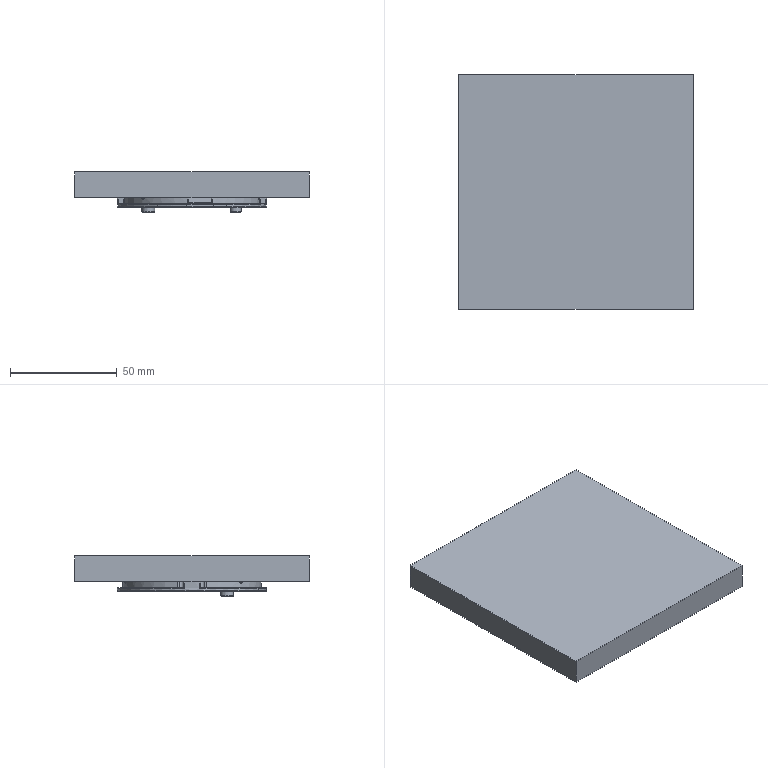NC program | NX | posted with a generic post | part box 110 x 110 x 18.8 mm
Lines 1 to 1769 of 9447:
N10 G17 G21 G94 G90
(FLOOR_WALL , TOOL : D63)
N12 T03 M6
N14 G54
N16 G17 G0 G90 X-77.5 Y42.997 S6500 M3
N18 G43 Z30. H3
N20 Z3.
N22 G94 G1 Z0. F1250.
N24 X-74.5
N26 X74.5
N28 Y12.599
N30 X-74.5
N32 Y-17.8
N34 X74.5
N36 X77.5
N38 Z3.
N40 G0 Z30.
N42 M5
(CAVITY_MILL , TOOL : D10)
N44 T04 M6
N46 G54
N48 G17 G0 G90 X-49.996 Y-4.33 S9500 M3
N50 G43 Z30. H4
N52 Z0.52
N54 G94 G1 Z-0.98 F1000.
N56 X-43.996 Y-0.866
N58 G3 X-43.496 Y0. R1.
N60 G1 Y43.007 F3000.
N62 G2 X-43.007 Y43.496 R0.489
N64 G1 X43.007
N66 G2 X43.496 Y43.007 R0.489
N68 G1 Y-43.007
N70 G2 X43.007 Y-43.496 R0.489
N72 G1 X-43.007
N74 G2 X-43.496 Y-43.007 R0.489
N76 G1 Y0.
N78 X-37.496
N80 Y37.496
N82 X37.496
N84 Y-37.496
N86 X-37.496
N88 Y0.
N90 X-31.496
N92 Y31.496
N94 X31.496
N96 Y-31.496
N98 X-31.496
N100 Y0.
N102 X-25.496
N104 Y25.496
N106 X25.496
N108 Y24.657
N110 G3 X22.5 Y25.3 R7.3
N112 G1 X10.5
N114 G3 X3.2 Y18. R7.3
N116 G1 Y-18.
N118 G3 X10.5 Y-25.3 R7.3
N120 G1 X22.5
N122 G3 X25.496 Y-24.657 R7.3
N124 G1 X25.003 Y-23.563
N126 G2 X22.5 Y-24.1 R6.1
N128 G1 X10.5
N130 G2 X4.4 Y-18. R6.1
N132 G1 Y18.
N134 G2 X10.5 Y24.1 R6.1
N136 G1 X22.5
N138 G2 X28.6 Y18. R6.1
N140 G1 Y-18.
N142 G2 X25.003 Y-23.563 R6.1
N144 G1 X25.496 Y-24.657
N146 Y-25.496
N148 X-25.496
N150 Y0.
N152 X-19.496
N154 Y19.496
N156 X-2.716
N158 G3 X-2.8 Y18. R13.3
N160 G1 Y-18.
N162 G3 X-2.716 Y-19.496 R13.3
N164 G1 X-19.496
N166 Y0.
N168 X-13.496
N170 Y13.496
N172 X-8.8
N174 Y-13.496
N176 X-13.496
N178 Y0.
N180 G3 X-13.996 Y0.866 R1.
N182 G1 Z0.52
N184 G0 X-49.996 Y-4.33 Z-0.46
N186 G1 Z-1.96 F1000.
N188 X-43.996 Y-0.866
N190 G3 X-43.496 Y0. R1.
N192 G1 Y43.006 F3000.
N194 G2 X-43.006 Y43.496 R0.489
N196 G1 X43.006
N198 G2 X43.496 Y43.006 R0.489
N200 G1 Y-43.006
N202 G2 X43.006 Y-43.496 R0.489
N204 G1 X-43.006
N206 G2 X-43.496 Y-43.006 R0.489
N208 G1 Y0.
N210 X-37.496
N212 Y37.496
N214 X37.496
N216 Y-37.496
N218 X-37.496
N220 Y0.
N222 X-31.496
N224 Y31.496
N226 X31.496
N228 Y-31.496
N230 X-31.496
N232 Y0.
N234 X-25.496
N236 Y25.496
N238 X25.496
N240 Y24.657
N242 G3 X22.5 Y25.3 R7.3
N244 G1 X10.5
N246 G3 X3.2 Y18. R7.3
N248 G1 Y-18.
N250 G3 X10.5 Y-25.3 R7.3
N252 G1 X22.5
N254 G3 X25.496 Y-24.657 R7.3
N256 G1 X25.003 Y-23.563
N258 G2 X22.5 Y-24.1 R6.1
N260 G1 X10.5
N262 G2 X4.4 Y-18. R6.1
N264 G1 Y18.
N266 G2 X10.5 Y24.1 R6.1
N268 G1 X22.5
N270 G2 X28.6 Y18. R6.1
N272 G1 Y-18.
N274 G2 X25.003 Y-23.563 R6.1
N276 G1 X25.496 Y-24.657
N278 Y-25.496
N280 X-25.496
N282 Y0.
N284 X-19.496
N286 Y19.496
N288 X-2.716
N290 G3 X-2.8 Y18. R13.3
N292 G1 Y-18.
N294 G3 X-2.716 Y-19.496 R13.3
N296 G1 X-19.496
N298 Y0.
N300 X-13.496
N302 Y13.496
N304 X-8.8
N306 Y-13.496
N308 X-13.496
N310 Y0.
N312 G3 X-13.996 Y0.866 R1.
N314 G1 Z-0.46
N316 G0 X-49.996 Y-4.33 Z-1.44
N318 G1 Z-2.94 F1000.
N320 X-43.996 Y-0.866
N322 G3 X-43.496 Y0. R1.
N324 G1 Y43.006 F3000.
N326 G2 X-43.006 Y43.496 R0.49
N328 G1 X43.006
N330 G2 X43.496 Y43.006 R0.49
N332 G1 Y-43.006
N334 G2 X43.006 Y-43.496 R0.49
N336 G1 X-43.006
N338 G2 X-43.496 Y-43.006 R0.49
N340 G1 Y0.
N342 X-37.496
N344 Y37.496
N346 X37.496
N348 Y-37.496
N350 X-37.496
N352 Y0.
N354 X-31.496
N356 Y31.496
N358 X31.496
N360 Y-31.496
N362 X-31.496
N364 Y0.
N366 X-25.496
N368 Y25.496
N370 X25.496
N372 Y24.657
N374 G3 X22.5 Y25.3 R7.3
N376 G1 X10.5
N378 G3 X3.2 Y18. R7.3
N380 G1 Y-18.
N382 G3 X10.5 Y-25.3 R7.3
N384 G1 X22.5
N386 G3 X25.496 Y-24.657 R7.3
N388 G1 X25.004 Y-23.563
N390 G2 X22.5 Y-24.1 R6.1
N392 G1 X10.5
N394 G2 X4.4 Y-18. R6.1
N396 G1 Y18.
N398 G2 X10.5 Y24.1 R6.1
N400 G1 X22.5
N402 G2 X28.6 Y18. R6.1
N404 G1 Y-18.
N406 G2 X25.004 Y-23.563 R6.1
N408 G1 X25.496 Y-24.657
N410 Y-25.496
N412 X-25.496
N414 Y0.
N416 X-19.496
N418 Y19.496
N420 X-2.716
N422 G3 X-2.8 Y18. R13.3
N424 G1 Y-18.
N426 G3 X-2.716 Y-19.496 R13.3
N428 G1 X-19.496
N430 Y0.
N432 X-13.496
N434 Y13.496
N436 X-8.8
N438 Y-13.496
N440 X-13.496
N442 Y0.
N444 G3 X-13.996 Y0.866 R1.
N446 G1 Z-1.44
N448 G0 X-49.996 Y-4.33 Z-2.42
N450 G1 Z-3.92 F1000.
N452 X-43.996 Y-0.866
N454 G3 X-43.496 Y0. R1.
N456 G1 Y43.006 F3000.
N458 G2 X-43.006 Y43.496 R0.491
N460 G1 X43.006
N462 G2 X43.496 Y43.006 R0.491
N464 G1 Y-43.006
N466 G2 X43.006 Y-43.496 R0.491
N468 G1 X-43.006
N470 G2 X-43.496 Y-43.006 R0.491
N472 G1 Y0.
N474 X-37.496
N476 Y37.496
N478 X37.496
N480 Y-37.496
N482 X-37.496
N484 Y0.
N486 X-31.496
N488 Y31.496
N490 X31.496
N492 Y-31.496
N494 X-31.496
N496 Y0.
N498 X-25.496
N500 Y25.496
N502 X25.496
N504 Y24.657
N506 G3 X22.5 Y25.3 R7.3
N508 G1 X10.5
N510 G3 X3.2 Y18. R7.3
N512 G1 Y-18.
N514 G3 X10.5 Y-25.3 R7.3
N516 G1 X22.5
N518 G3 X25.496 Y-24.657 R7.3
N520 G1 X25.004 Y-23.562
N522 G2 X22.5 Y-24.1 R6.1
N524 G1 X10.5
N526 G2 X4.4 Y-18. R6.1
N528 G1 Y18.
N530 G2 X10.5 Y24.1 R6.1
N532 G1 X22.5
N534 G2 X28.6 Y18. R6.1
N536 G1 Y-18.
N538 G2 X25.004 Y-23.562 R6.1
N540 G1 X25.496 Y-24.657
N542 Y-25.496
N544 X-25.496
N546 Y0.
N548 X-19.496
N550 Y19.496
N552 X-2.716
N554 G3 X-2.8 Y18. R13.3
N556 G1 Y-18.
N558 G3 X-2.716 Y-19.496 R13.3
N560 G1 X-19.496
N562 Y0.
N564 X-13.496
N566 Y13.496
N568 X-8.8
N570 Y-13.496
N572 X-13.496
N574 Y0.
N576 G3 X-13.996 Y0.866 R1.
N578 G1 Z-2.42
N580 G0 X-49.997 Y-4.33 Z-3.4
N582 G1 Z-4.9 F1000.
N584 X-43.997 Y-0.866
N586 G3 X-43.497 Y0. R1.
N588 G1 Y43.006 F3000.
N590 G2 X-43.006 Y43.497 R0.491
N592 G1 X43.006
N594 G2 X43.497 Y43.006 R0.491
N596 G1 Y-43.006
N598 G2 X43.006 Y-43.497 R0.491
N600 G1 X-43.006
N602 G2 X-43.497 Y-43.006 R0.491
N604 G1 Y0.
N606 X-37.497
N608 Y37.497
N610 X37.497
N612 Y-37.497
N614 X-37.497
N616 Y0.
N618 X-31.497
N620 Y31.497
N622 X31.497
N624 Y-31.497
N626 X-31.497
N628 Y0.
N630 X-25.497
N632 Y25.497
N634 X25.497
N636 Y24.657
N638 G3 X22.5 Y25.3 R7.3
N640 G1 X10.5
N642 G3 X3.2 Y18. R7.3
N644 G1 Y-18.
N646 G3 X10.5 Y-25.3 R7.3
N648 G1 X22.5
N650 G3 X25.497 Y-24.657 R7.3
N652 G1 X25.004 Y-23.562
N654 G2 X22.5 Y-24.1 R6.1
N656 G1 X10.5
N658 G2 X4.4 Y-18. R6.1
N660 G1 Y18.
N662 G2 X10.5 Y24.1 R6.1
N664 G1 X22.5
N666 G2 X28.6 Y18. R6.1
N668 G1 Y-18.
N670 G2 X25.004 Y-23.562 R6.1
N672 G1 X25.497 Y-24.657
N674 Y-25.497
N676 X-25.497
N678 Y0.
N680 X-19.497
N682 Y19.497
N684 X-2.716
N686 G3 X-2.8 Y18. R13.3
N688 G1 Y-18.
N690 G3 X-2.716 Y-19.497 R13.3
N692 G1 X-19.497
N694 Y0.
N696 X-13.497
N698 Y13.497
N700 X-8.8
N702 Y-13.497
N704 X-13.497
N706 Y0.
N708 G3 X-13.997 Y0.866 R1.
N710 G1 Z-3.4
N712 G0 X-49.997 Y-4.33 Z-4.4
N714 G1 Z-5.9 F1000.
N716 X-43.997 Y-0.866
N718 G3 X-43.497 Y0. R1.
N720 G1 Y43.005 F3000.
N722 G2 X-43.005 Y43.497 R0.492
N724 G1 X43.005
N726 G2 X43.497 Y43.005 R0.492
N728 G1 Y9.575
N730 X37.497
N732 G3 X9.575 Y37.497 R38.7
N734 G1 X4.435 Y38.471
N736 X9.575 Y37.497
N738 X37.497
N740 Y27.883
N742 X32.997
N744 G3 X27.883 Y32.997 R43.2
N746 G1 X32.997
N748 Y27.883
N750 X37.497
N752 Y9.575
N754 X43.497
N756 Y-43.005
N758 G2 X43.005 Y-43.497 R0.492
N760 G1 X-43.005
N762 G2 X-43.497 Y-43.005 R0.492
N764 G1 Y0.
N766 X-37.497 Y-9.575
N768 G3 X-13.805 Y-36.154 R38.7
N770 X-4.989 Y-32.127 R6.8
N772 G1 X-4.647 Y-31.187
N774 G3 X-8.608 Y-22.51 R6.8
N776 G2 X-11.58 Y-21.136 R24.1
N778 G3 X-14.058 Y-17.182 R7.3
N780 G2 X-17.182 Y-14.058 R22.2
N782 G3 X-21.136 Y-11.58 R7.3
N784 G2 X-11.287 Y21.293 R24.1
N786 G3 X-8.413 Y30.389 R6.8
N788 G1 X-8.867 Y31.28
N790 G3 X-18.108 Y34.202 R6.8
N792 X-37.497 Y9.575 R38.7
N794 G1 X-36.334 Y9.278
N796 G2 X-17.546 Y33.142 R37.5
N798 X-9.936 Y30.735 R5.6
N800 G1 X-9.482 Y29.844
N802 G2 X-11.849 Y22.354 R5.6
N804 G3 X-21.91 Y-12.65 R25.3
N806 G2 X-18.111 Y-14.817 R6.1
N808 G3 X-14.817 Y-18.111 R23.4
N810 G2 X-12.65 Y-21.91 R6.1
N812 G3 X-9.037 Y-23.631 R25.3
N814 G2 X-5.775 Y-30.777 R5.6
N816 G1 X-6.117 Y-31.717
N818 G2 X-13.377 Y-35.033 R5.6
N820 X-36.709 Y-7.66 R37.5
N822 X-36.799 Y-5.723 R6.1
N824 X-37.302 Y-3.849 R6.1
N826 X-37.302 Y3.849 R37.5
N828 X-36.799 Y5.723 R6.1
N830 X-36.709 Y7.66 R6.1
N832 X-36.334 Y9.278 R37.5
N834 G1 X-37.497 Y9.575
N836 Y37.497
N838 X-29.217
N840 X-31.423 Y31.423
N842 X-29.217 Y37.497
N844 X-4.467
N846 G3 X-7.409 Y31.657 R6.8
N848 G1 X-7.374 Y30.657
N850 G3 X-0.451 Y24.096 R6.8
N852 G2 X5.626 Y23.434 R24.1
N854 G3 X3.2 Y18. R7.3
N856 G1 Y-18.
N858 G3 X3.225 Y-18.605 R7.3
N860 G1 X-2.754 Y-19.103
N862 G3 X-6.465 Y-16.906 R12.8
N864 G2 X-6.85 Y-16.754 R18.1
N866 G3 X-10.258 Y-12.538 R13.3
N868 G2 X-12.538 Y-10.258 R16.2
N870 G3 X-16.754 Y-6.85 R13.3
N872 G2 X-8.477 Y15.992 R18.1
N874 G3 X-4.871 Y18.836 R12.8
N876 X-2.797 Y18.288 R12.8
N878 X-2.8 Y18. R13.3
N880 G1 Y-18.
N882 G3 X-2.754 Y-19.103 R13.3
N884 G1 X-8.8 Y-5.429
N886 G3 X-11.753 Y-2.877 R19.3
N888 G2 X-8.8 Y8.305 R12.1
N890 G1 Y-5.429
N892 X-2.754 Y-19.103
N894 X3.225 Y-18.605
N896 G3 X9.211 Y-25.185 R7.3
N898 X9.992 Y-29.907 R6.8
N900 G1 X10.492 Y-30.773
N902 G3 X19.873 Y-33.208 R6.8
N904 X25.874 Y-28.779 R38.7
N906 G1 X31.423 Y-31.423
N908 X25.874 Y-28.779
N910 G3 X37.497 Y-9.575 R38.7
N912 G1 X36.334 Y-9.278
N914 G2 X19.257 Y-32.178 R37.5
N916 X11.531 Y-30.173 R5.6
N918 G1 X11.031 Y-29.307
N920 G2 X10.827 Y-24.1 R5.6
N922 G1 X10.5
N924 G2 X4.4 Y-18. R6.1
N926 G1 Y18.
N928 G2 X8.598 Y23.796 R6.1
N930 G1 X8.528 Y23.82
N932 G3 X-0.474 Y25.296 R25.3
N934 G2 X-6.175 Y30.699 R5.6
N936 G1 X-6.21 Y31.699
N938 G2 X-0.721 Y37.493 R5.6
N940 X36.709 Y7.66 R37.5
N942 X36.799 Y5.722 R6.1
N944 X37.302 Y3.849 R6.1
N946 X37.302 Y-3.849 R37.5
N948 X36.799 Y-5.723 R6.1
N950 X36.709 Y-7.66 R6.1
N952 X36.334 Y-9.278 R37.5
N954 G1 X37.497 Y-9.575
N956 Y-37.497
N958 X1.489
N960 Y-31.497
N962 G3 X1.734 Y-28.003 R12.8
N964 X3.374 Y-29.23 R13.3
N966 X4.094 Y-31.497 R12.8
N968 G1 X1.489
N970 Y-37.497
N972 X-32.497
N974 X-31.423 Y-31.423
N976 X-32.497 Y-37.497
N978 X-37.497
N980 Y-9.575
N982 G3 X-37.997 Y-8.709 R1.
N984 G1 X-49.997
N986 Z-4.4
N988 G0 Y-4.33 Z-5.4
N990 G1 Z-6.9 F1000.
N992 X-43.997 Y-0.866
N994 G3 X-43.497 Y0. R1.
N996 G1 Y43.005 F3000.
N998 G2 X-43.005 Y43.497 R0.492
N1000 G1 X-9.574
N1002 Y37.497
N1004 G3 X-37.497 Y9.574 R38.7
N1006 G1 Y37.497
N1008 X-27.882
N1010 Y32.997
N1012 G3 X-32.997 Y27.882 R43.2
N1014 G1 Y32.997
N1016 X-27.882
N1018 Y37.497
N1020 X-9.574
N1022 X-4.434 Y38.471
N1024 X-9.574 Y37.497
N1026 Y43.497
N1028 X43.005
N1030 G2 X43.497 Y43.005 R0.492
N1032 G1 Y9.574
N1034 X37.497
N1036 G3 X9.574 Y37.497 R38.7
N1038 G1 X4.434 Y38.471
N1040 X9.574 Y37.497
N1042 X37.497
N1044 Y27.882
N1046 X32.997
N1048 G3 X27.882 Y32.997 R43.2
N1050 G1 X32.997
N1052 Y27.882
N1054 X37.497
N1056 Y9.574
N1058 X43.497
N1060 Y-43.005
N1062 G2 X43.005 Y-43.497 R0.492
N1064 G1 X-43.005
N1066 G2 X-43.497 Y-43.005 R0.492
N1068 G1 Y-9.574
N1070 X-37.497
N1072 G3 X-13.805 Y-36.154 R38.7
N1074 X-4.989 Y-32.127 R6.8
N1076 G1 X-4.647 Y-31.187
N1078 G3 X-8.608 Y-22.51 R6.8
N1080 G2 X-11.58 Y-21.136 R24.1
N1082 G3 X-14.058 Y-17.182 R7.3
N1084 G2 X-17.182 Y-14.058 R22.2
N1086 G3 X-21.136 Y-11.58 R7.3
N1088 G2 X-12.514 Y20.596 R24.1
N1090 G3 X-7.851 Y20.765 R7.3
N1092 G2 X-3.583 Y21.909 R22.2
N1094 G3 X0.539 Y24.094 R7.3
N1096 G2 X5.626 Y23.434 R24.1
N1098 G3 X3.2 Y18. R7.3
N1100 G1 Y-18.
N1102 G3 X3.225 Y-18.605 R7.3
N1104 G1 X-2.754 Y-19.103
N1106 G3 X-6.465 Y-16.906 R12.8
N1108 G2 X-6.85 Y-16.754 R18.1
N1110 G3 X-10.258 Y-12.538 R13.3
N1112 G2 X-12.538 Y-10.258 R16.2
N1114 G3 X-16.754 Y-6.85 R13.3
N1116 G2 X-11.084 Y14.309 R18.1
N1118 G3 X-5.729 Y15.153 R13.3
N1120 G2 X-2.8 Y15.956 R16.2
N1122 G1 Y-18.
N1124 G3 X-2.754 Y-19.103 R13.3
N1126 G1 X-8.8 Y-5.429
N1128 G3 X-11.753 Y-2.877 R19.3
N1130 G2 X-8.8 Y8.305 R12.1
N1132 G1 Y-5.429
N1134 X-2.754 Y-19.103
N1136 X3.225 Y-18.605
N1138 G3 X9.211 Y-25.185 R7.3
N1140 X9.992 Y-29.907 R6.8
N1142 G1 X10.492 Y-30.773
N1144 G3 X19.873 Y-33.208 R6.8
N1146 X25.874 Y-28.779 R38.7
N1148 G1 X31.423 Y-31.423
N1150 X25.874 Y-28.779
N1152 G3 X37.497 Y-9.574 R38.7
N1154 G1 X36.334 Y-9.277
N1156 G2 X19.257 Y-32.178 R37.5
N1158 X11.531 Y-30.173 R5.6
N1160 G1 X11.031 Y-29.307
N1162 G2 X10.825 Y-24.1 R5.6
N1164 G1 X10.5
N1166 G2 X4.4 Y-18. R6.1
N1168 G1 Y18.
N1170 G2 X8.598 Y23.796 R6.1
N1172 G1 X8.528 Y23.82
N1174 G3 X0. Y25.3 R25.3
N1176 G2 X-3.777 Y23.093 R6.1
N1178 G3 X-8.276 Y21.888 R23.4
N1180 G2 X-12.65 Y21.911 R6.1
N1182 G3 X-21.91 Y-12.65 R25.3
N1184 G2 X-18.111 Y-14.817 R6.1
N1186 G3 X-14.817 Y-18.111 R23.4
N1188 G2 X-12.65 Y-21.91 R6.1
N1190 G3 X-9.037 Y-23.631 R25.3
N1192 G2 X-5.775 Y-30.777 R5.6
N1194 G1 X-6.117 Y-31.717
N1196 G2 X-13.377 Y-35.033 R5.6
N1198 X-36.709 Y-7.66 R37.5
N1200 X-36.799 Y-5.723 R6.1
N1202 X-37.302 Y-3.849 R6.1
N1204 X-37.302 Y3.849 R37.5
N1206 X-36.799 Y5.723 R6.1
N1208 X-36.709 Y7.66 R6.1
N1210 X36.709 Y7.66 R37.5
N1212 X36.799 Y5.722 R6.1
N1214 X37.302 Y3.849 R6.1
N1216 X37.302 Y-3.849 R37.5
N1218 X36.799 Y-5.723 R6.1
N1220 X36.709 Y-7.66 R6.1
N1222 X36.334 Y-9.277 R37.5
N1224 G1 X37.497 Y-9.574
N1226 Y-37.497
N1228 X1.489
N1230 Y-31.497
N1232 G3 X1.734 Y-28.003 R12.8
N1234 X3.374 Y-29.23 R13.3
N1236 X4.094 Y-31.497 R12.8
N1238 G1 X1.489
N1240 Y-37.497
N1242 X-32.497
N1244 X-31.423 Y-31.423
N1246 X-32.497 Y-37.497
N1248 X-37.497
N1250 Y-9.574
N1252 X-43.497
N1254 Y0.
N1256 G3 X-43.997 Y0.866 R1.
N1258 G1 X-49.997 Y4.33
N1260 Z-5.4
N1262 G0 Y-4.33 Z-6.4
N1264 G1 Z-7.9 F1000.
N1266 X-43.997 Y-0.866
N1268 G3 X-43.497 Y0. R1.
N1270 G1 Y43.005 F3000.
N1272 G2 X-43.005 Y43.497 R0.493
N1274 G1 X-9.573
N1276 Y37.497
N1278 G3 X-37.497 Y9.573 R38.7
N1280 G1 Y37.497
N1282 X-27.882
N1284 Y32.997
N1286 G3 X-32.997 Y27.882 R43.2
N1288 G1 Y32.997
N1290 X-27.882
N1292 Y37.497
N1294 X-9.573
N1296 X-4.432 Y38.471
N1298 X-9.573 Y37.497
N1300 Y43.497
N1302 X43.005
N1304 G2 X43.497 Y43.005 R0.493
N1306 G1 Y9.573
N1308 X37.497
N1310 G3 X9.573 Y37.497 R38.7
N1312 G1 X4.432 Y38.471
N1314 X9.573 Y37.497
N1316 X37.497
N1318 Y27.882
N1320 X32.997
N1322 G3 X27.882 Y32.997 R43.2
N1324 G1 X32.997
N1326 Y27.882
N1328 X37.497
N1330 Y9.573
N1332 X43.497
N1334 Y-43.005
N1336 G2 X43.005 Y-43.497 R0.493
N1338 G1 X-43.005
N1340 G2 X-43.497 Y-43.005 R0.493
N1342 G1 Y0.
N1344 X-37.497 Y-9.573
N1346 G3 X-13.805 Y-36.154 R38.7
N1348 X-4.989 Y-32.127 R6.8
N1350 G1 X-4.647 Y-31.187
N1352 G3 X-8.608 Y-22.51 R6.8
N1354 G2 X-11.58 Y-21.136 R24.1
N1356 G3 X-14.058 Y-17.182 R7.3
N1358 G2 X-17.182 Y-14.058 R22.2
N1360 G3 X-21.136 Y-11.58 R7.3
N1362 G2 X-12.514 Y20.596 R24.1
N1364 G3 X-7.851 Y20.765 R7.3
N1366 G2 X-3.583 Y21.909 R22.2
N1368 G3 X0.539 Y24.094 R7.3
N1370 G2 X5.626 Y23.434 R24.1
N1372 G3 X3.2 Y18. R7.3
N1374 G1 Y-18.
N1376 G3 X3.225 Y-18.605 R7.3
N1378 G1 X-2.754 Y-19.103
N1380 G3 X-6.465 Y-16.906 R12.8
N1382 G2 X-6.85 Y-16.754 R18.1
N1384 G3 X-10.258 Y-12.538 R13.3
N1386 G2 X-12.538 Y-10.258 R16.2
N1388 G3 X-16.754 Y-6.85 R13.3
N1390 G2 X-11.084 Y14.309 R18.1
N1392 G3 X-5.729 Y15.153 R13.3
N1394 G2 X-2.8 Y15.956 R16.2
N1396 G1 Y-18.
N1398 G3 X-2.754 Y-19.103 R13.3
N1400 G1 X-8.8 Y-5.429
N1402 G3 X-11.753 Y-2.877 R19.3
N1404 G2 X-8.8 Y8.305 R12.1
N1406 G1 Y-5.429
N1408 X-2.754 Y-19.103
N1410 X3.225 Y-18.605
N1412 G3 X9.211 Y-25.185 R7.3
N1414 X9.992 Y-29.907 R6.8
N1416 G1 X10.492 Y-30.773
N1418 G3 X19.873 Y-33.208 R6.8
N1420 X37.497 Y-9.573 R38.7
N1422 G1 X36.335 Y-9.276
N1424 G2 X19.257 Y-32.178 R37.5
N1426 X11.531 Y-30.173 R5.6
N1428 G1 X11.031 Y-29.307
N1430 G2 X10.823 Y-24.1 R5.601
N1432 G1 X10.5
N1434 G2 X4.4 Y-18. R6.1
N1436 G1 Y18.
N1438 G2 X8.597 Y23.795 R6.1
N1440 G1 X8.528 Y23.82
N1442 G3 X0. Y25.3 R25.3
N1444 G2 X-3.777 Y23.093 R6.1
N1446 G3 X-8.276 Y21.888 R23.4
N1448 G2 X-12.65 Y21.911 R6.1
N1450 G3 X-21.91 Y-12.65 R25.3
N1452 G2 X-18.111 Y-14.817 R6.1
N1454 G3 X-14.817 Y-18.111 R23.4
N1456 G2 X-12.65 Y-21.91 R6.1
N1458 G3 X-9.037 Y-23.631 R25.3
N1460 G2 X-5.775 Y-30.777 R5.6
N1462 G1 X-6.117 Y-31.717
N1464 G2 X-13.377 Y-35.033 R5.6
N1466 X-36.709 Y-7.66 R37.5
N1468 X-36.799 Y-5.723 R6.1
N1470 X-37.302 Y-3.849 R6.1
N1472 X-37.302 Y3.849 R37.5
N1474 X-36.799 Y5.723 R6.1
N1476 X-36.709 Y7.66 R6.1
N1478 X36.709 Y7.66 R37.5
N1480 X36.799 Y5.722 R6.1
N1482 X37.302 Y3.849 R6.1
N1484 X37.302 Y-3.849 R37.5
N1486 X36.799 Y-5.723 R6.1
N1488 X36.709 Y-7.66 R6.1
N1490 X36.335 Y-9.276 R37.5
N1492 G1 X37.497 Y-9.573
N1494 Y-37.497
N1496 X29.217
N1498 X31.423 Y-31.423
N1500 X29.217 Y-37.497
N1502 X1.489
N1504 Y-31.497
N1506 G3 X1.734 Y-28.003 R12.8
N1508 X3.374 Y-29.23 R13.3
N1510 X4.094 Y-31.497 R12.8
N1512 G1 X1.489
N1514 Y-37.497
N1516 X-37.497
N1518 Y-32.497
N1520 X-31.423 Y-31.423
N1522 X-37.497 Y-32.497
N1524 Y-9.573
N1526 G3 X-37.997 Y-8.707 R1.
N1528 G1 X-49.997
N1530 Z-6.4
N1532 G0 X-49.998 Y-4.33 Z-7.4
N1534 G1 Z-8.9 F1000.
N1536 X-43.998 Y-0.866
N1538 G3 X-43.498 Y0. R1.
N1540 G1 Y43.004 F3000.
N1542 G2 X-43.004 Y43.498 R0.493
N1544 G1 X-9.572
N1546 Y37.498
N1548 G3 X-37.498 Y9.572 R38.7
N1550 G1 Y37.498
N1552 X-27.882
N1554 Y32.998
N1556 G3 X-32.998 Y27.882 R43.2
N1558 G1 Y32.998
N1560 X-27.882
N1562 Y37.498
N1564 X-9.572
N1566 X-4.431 Y38.472
N1568 X-9.572 Y37.498
N1570 Y43.498
N1572 X43.004
N1574 G2 X43.498 Y43.004 R0.493
N1576 G1 Y9.572
N1578 X37.498
N1580 G3 X9.572 Y37.498 R38.7
N1582 G1 X4.431 Y38.472
N1584 X9.572 Y37.498
N1586 X37.498
N1588 Y27.882
N1590 X32.998
N1592 G3 X27.882 Y32.998 R43.2
N1594 G1 X32.998
N1596 Y27.882
N1598 X37.498
N1600 Y9.572
N1602 X43.498
N1604 Y-43.004
N1606 G2 X43.004 Y-43.498 R0.493
N1608 G1 X-43.004
N1610 G2 X-43.498 Y-43.004 R0.493
N1612 G1 Y0.
N1614 X-37.498 Y-9.572
N1616 G3 X-13.805 Y-36.154 R38.7
N1618 X-4.989 Y-32.127 R6.8
N1620 G1 X-4.647 Y-31.187
N1622 G3 X-8.608 Y-22.51 R6.8
N1624 G2 X-11.58 Y-21.136 R24.1
N1626 G3 X-14.058 Y-17.182 R7.3
N1628 G2 X-17.182 Y-14.058 R22.2
N1630 G3 X-21.136 Y-11.58 R7.3
N1632 G2 X-12.514 Y20.596 R24.1
N1634 G3 X-7.851 Y20.765 R7.3
N1636 G2 X-3.583 Y21.909 R22.2
N1638 G3 X0.539 Y24.094 R7.3
N1640 G2 X5.626 Y23.434 R24.1
N1642 G3 X3.2 Y18. R7.3
N1644 G1 Y-18.
N1646 G3 X3.225 Y-18.605 R7.3
N1648 G1 X-2.754 Y-19.103
N1650 G3 X-6.465 Y-16.906 R12.8
N1652 G2 X-6.85 Y-16.754 R18.1
N1654 G3 X-10.258 Y-12.538 R13.3
N1656 G2 X-12.538 Y-10.258 R16.2
N1658 G3 X-16.754 Y-6.85 R13.3
N1660 G2 X-11.084 Y14.309 R18.1
N1662 G3 X-5.729 Y15.153 R13.3
N1664 G2 X-2.8 Y15.956 R16.2
N1666 G1 Y-18.
N1668 G3 X-2.754 Y-19.103 R13.3
N1670 G1 X-8.8 Y-5.429
N1672 G3 X-11.753 Y-2.877 R19.3
N1674 G2 X-8.8 Y8.305 R12.1
N1676 G1 Y-5.429
N1678 X-2.754 Y-19.103
N1680 X3.225 Y-18.605
N1682 G3 X9.211 Y-25.185 R7.3
N1684 X9.992 Y-29.907 R6.8
N1686 G1 X10.492 Y-30.773
N1688 G3 X19.873 Y-33.208 R6.8
N1690 X25.874 Y-28.779 R38.7
N1692 G1 X31.423 Y-31.423
N1694 X25.874 Y-28.779
N1696 G3 X37.498 Y-9.572 R38.7
N1698 G1 X36.335 Y-9.275
N1700 G2 X19.257 Y-32.178 R37.5
N1702 X11.531 Y-30.173 R5.6
N1704 G1 X11.031 Y-29.307
N1706 G2 X10.822 Y-24.1 R5.602
N1708 G1 X10.5
N1710 G2 X4.4 Y-18. R6.1
N1712 G1 Y18.
N1714 G2 X8.596 Y23.795 R6.1
N1716 G1 X8.528 Y23.82
N1718 G3 X0. Y25.3 R25.3
N1720 G2 X-3.777 Y23.093 R6.1
N1722 G3 X-8.276 Y21.888 R23.4
N1724 G2 X-12.65 Y21.911 R6.1
N1726 G3 X-21.91 Y-12.65 R25.3
N1728 G2 X-18.111 Y-14.817 R6.1
N1730 G3 X-14.817 Y-18.111 R23.4
N1732 G2 X-12.65 Y-21.91 R6.1
N1734 G3 X-9.037 Y-23.631 R25.3
N1736 G2 X-5.775 Y-30.777 R5.6
N1738 G1 X-6.117 Y-31.717
N1740 G2 X-13.377 Y-35.033 R5.6
N1742 X-36.709 Y-7.66 R37.5
N1744 X-36.799 Y-5.723 R6.1
N1746 X-37.302 Y-3.849 R6.1
N1748 X-37.302 Y3.849 R37.5
N1750 X-36.799 Y5.723 R6.1
N1752 X-36.709 Y7.66 R6.1
N1754 X36.709 Y7.66 R37.5
N1756 X36.799 Y5.722 R6.1
N1758 X37.302 Y3.849 R6.1
N1760 X37.302 Y-3.849 R37.5
N1762 X36.799 Y-5.723 R6.1
N1764 X36.709 Y-7.66 R6.1
N1766 X36.335 Y-9.275 R37.5
N1768 G1 X37.498 Y-9.572
N1770 Y-37.498
N1772 X1.489
N1774 Y-31.498
N1776 G3 X1.734 Y-28.003 R12.8
N1778 X3.374 Y-29.23 R13.3
N1780 X4.094 Y-31.498 R12.8
N1782 G1 X1.489
N1784 Y-37.498
N1786 X-32.498
N1788 X-31.423 Y-31.423
N1790 X-32.498 Y-37.498
N1792 X-37.498
N1794 Y-9.572
N1796 G3 X-37.998 Y-8.706 R1.
N1798 G1 X-49.998
N1800 Z-7.4
N1802 G0 Z30.
N1804 X34.77 Y-49.998
N1806 Z-8.233
N1808 G1 Z-9.733 F1000.
N1810 X31.306 Y-43.998
N1812 G3 X30.44 Y-43.498 R1.
N1814 G1 X-43.004 F3000.
N1816 G2 X-43.498 Y-43.004 R0.494
N1818 G1 Y-9.571
N1820 X-37.498
N1822 G3 X-9.571 Y-37.498 R38.7
N1824 G1 X-4.43 Y-38.472
N1826 X-9.571 Y-37.498
N1828 X-37.498
N1830 Y-27.882
N1832 X-32.998
N1834 G3 X-27.882 Y-32.998 R43.2
N1836 G1 X-32.998
N1838 Y-27.882
N1840 X-37.498
N1842 Y-9.571
N1844 X-43.498
N1846 Y43.004
N1848 G2 X-43.004 Y43.498 R0.494
N1850 G1 X-9.571
N1852 Y37.498
N1854 G3 X-37.498 Y9.571 R38.7
N1856 G1 Y37.498
N1858 X-27.882
N1860 Y32.998
N1862 G3 X-32.998 Y27.882 R43.2
N1864 G1 Y32.998
N1866 X-27.882
N1868 Y37.498
N1870 X-9.571
N1872 X-4.43 Y38.472
N1874 X-9.571 Y37.498
N1876 Y43.498
N1878 X43.004
N1880 G2 X43.498 Y43.004 R0.494
N1882 G1 Y9.571
N1884 X37.498
N1886 G3 X9.571 Y37.498 R38.7
N1888 G1 X4.43 Y38.472
N1890 X9.571 Y37.498
N1892 X37.498
N1894 Y27.882
N1896 X32.998
N1898 G3 X27.882 Y32.998 R43.2
N1900 G1 X32.998
N1902 Y27.882
N1904 X37.498
N1906 Y9.571
N1908 X43.498
N1910 Y-43.004
N1912 G2 X43.004 Y-43.498 R0.494
N1914 G1 X30.44
N1916 Y-37.498
N1918 X1.768
N1920 G3 X4.176 Y-34.683 R6.8
N1922 X11.525 Y-36.944 R6.8
N1924 X37.498 Y-9.571 R38.7
N1926 G1 X36.335 Y-9.274
N1928 G2 X11.168 Y-35.798 R37.5
N1930 X3.9 Y-30.453 R5.6
N1932 G1 Y-29.403
N1934 G2 X7.778 Y-24.075 R5.6
N1936 G3 X8.596 Y-23.795 R25.3
N1938 G2 X4.4 Y-18. R6.1
N1940 G1 Y18.
N1942 G2 X8.596 Y23.795 R6.1
N1944 G3 X0. Y25.3 R25.3
N1946 G2 X-3.777 Y23.093 R6.1
N1948 G3 X-8.276 Y21.888 R23.4
N1950 G2 X-12.65 Y21.911 R6.1
N1952 G3 X-21.91 Y-12.65 R25.3
N1954 G2 X-18.111 Y-14.817 R6.1
N1956 G3 X-14.817 Y-18.111 R23.4
N1958 G2 X-12.65 Y-21.91 R6.1
N1960 G3 X-1.638 Y-25.247 R25.3
N1962 G2 X3.6 Y-30.835 R5.6
N1964 G1 Y-31.837
N1966 G2 X-2.351 Y-37.426 R5.6
N1968 X-36.485 Y-8.665 R37.5
N1970 X-39.893 Y-4.068 R5.6
N1972 X-39.893 Y4.068 R40.1
N1974 X-36.485 Y8.665 R5.6
N1976 X36.485 Y8.665 R37.5
N1978 X39.893 Y4.068 R5.6
N1980 X39.893 Y-4.068 R40.1
N1982 X36.485 Y-8.665 R5.6
N1984 X36.335 Y-9.274 R37.5
N1986 G1 X37.498 Y-9.571
N1988 Y-37.498
N1990 X30.44
N1992 Y-32.998
N1994 X27.882
N1996 G3 X32.998 Y-27.882 R43.2
N1998 G1 Y-32.998
N2000 X30.44
N2002 G3 X29.574 Y-33.498 R1.
N2004 G1 Z-8.233
N2006 G0 Z30.
N2008 X-14.756 Y19.055
N2010 Z-7.4
N2012 G1 X-13.807 Y19.789 Z-7.463 F1000.
N2014 X-13.542 Y19.972 Z-7.48
N2016 X-12.514 Y20.596 Z-7.543
N2018 X-11.879 Y20.408 Z-7.578
N2020 X-11.452 Y20.335 Z-7.6
N2022 X-10.128 Y20.27 Z-7.67
N2024 X-8.471 Y20.531 Z-7.758
N2026 X-6.771 Y21.174 Z-7.853
N2028 X-4.974 Y21.666 Z-7.95
N2030 X-3.71 Y21.888 Z-8.018
N2032 X-2.929 Y22.016 Z-8.059
N2034 X-1.329 Y22.637 Z-8.149
N2036 X0.084 Y23.613 Z-8.239
N2038 X0.539 Y24.094 Z-8.274
N2040 X1.742 Y24.067 Z-8.337
N2042 X4.456 Y23.715 Z-8.48
N2044 X5.626 Y23.434 Z-8.543
N2046 X5.132 Y22.992 Z-8.578
N2048 X4.174 Y21.703 Z-8.662
N2050 X3.52 Y20.236 Z-8.746
N2052 X3.2 Y18.662 Z-8.831
N2054 Y1.438 Z-9.733
N2056 Y-18. F3000.
N2058 G3 X5.877 Y-23.649 R7.3
N2060 X3.31 Y-26.588 R6.8
N2062 X-1.56 Y-24.049 R6.8
N2064 G2 X-11.58 Y-21.136 R24.1
N2066 G3 X-14.058 Y-17.182 R7.3
N2068 G2 X-17.182 Y-14.058 R22.2
N2070 G3 X-21.136 Y-11.58 R7.3
N2072 G2 X-12.514 Y20.596 R24.1
N2074 G3 X-7.851 Y20.765 R7.3
N2076 G2 X-3.583 Y21.909 R22.2
N2078 G3 X0.539 Y24.094 R7.3
N2080 G2 X5.626 Y23.434 R24.1
N2082 G3 X3.2 Y18. R7.3
N2084 G1 Y1.438
N2086 X-2.8
N2088 Y-17.882
N2090 G2 X-6.85 Y-16.754 R18.1
N2092 G3 X-10.258 Y-12.538 R13.3
N2094 G2 X-12.538 Y-10.258 R16.2
N2096 G3 X-16.754 Y-6.85 R13.3
N2098 G2 X-11.084 Y14.309 R18.1
N2100 G3 X-5.729 Y15.153 R13.3
N2102 G2 X-2.8 Y15.956 R16.2
N2104 G1 Y1.438
N2106 X-8.8
N2108 Y-5.429
N2110 G3 X-11.753 Y-2.877 R19.3
N2112 G2 X-8.8 Y8.305 R12.1
N2114 G1 Y1.438
N2116 G3 X-8.3 Y0.572 R1.
N2118 G1 Z-8.233
N2120 G0 Z30.
N2122 X34.77 Y-49.998
N2124 Z-9.067
N2126 G1 Z-10.567 F1000.
N2128 X31.306 Y-43.998
N2130 G3 X30.44 Y-43.498 R1.
N2132 G1 X-43.004 F3000.
N2134 G2 X-43.498 Y-43.004 R0.494
N2136 G1 Y-9.57
N2138 X-37.498
N2140 G3 X-9.57 Y-37.498 R38.7
N2142 G1 X-4.428 Y-38.472
N2144 X-9.57 Y-37.498
N2146 X-37.498
N2148 Y-27.881
N2150 X-32.998
N2152 G3 X-27.881 Y-32.998 R43.2
N2154 G1 X-32.998
N2156 Y-27.881
N2158 X-37.498
N2160 Y-9.57
N2162 X-43.498
N2164 Y43.004
N2166 G2 X-43.004 Y43.498 R0.494
N2168 G1 X-9.57
N2170 Y37.498
N2172 G3 X-37.498 Y9.57 R38.7
N2174 G1 Y37.498
N2176 X-27.881
N2178 Y32.998
N2180 G3 X-32.998 Y27.881 R43.2
N2182 G1 Y32.998
N2184 X-27.881
N2186 Y37.498
N2188 X-9.57
N2190 X-4.428 Y38.472
N2192 X-9.57 Y37.498
N2194 Y43.498
N2196 X43.004
N2198 G2 X43.498 Y43.004 R0.494
N2200 G1 Y9.57
N2202 X37.498
N2204 G3 X9.57 Y37.498 R38.7
N2206 G1 X4.428 Y38.472
N2208 X9.57 Y37.498
N2210 X37.498
N2212 Y27.881
N2214 X32.998
N2216 G3 X27.881 Y32.998 R43.2
N2218 G1 X32.998
N2220 Y27.881
N2222 X37.498
N2224 Y9.57
N2226 X43.498
N2228 Y-43.004
N2230 G2 X43.004 Y-43.498 R0.494
N2232 G1 X30.44
N2234 Y-37.498
N2236 X1.768
N2238 G3 X4.176 Y-34.683 R6.8
N2240 X11.525 Y-36.944 R6.8
N2242 X37.498 Y-9.57 R38.7
N2244 G1 X36.335 Y-9.273
N2246 G2 X11.168 Y-35.798 R37.5
N2248 X3.9 Y-30.453 R5.6
N2250 G1 Y-29.403
N2252 G2 X7.778 Y-24.075 R5.6
N2254 G3 X8.596 Y-23.795 R25.3
N2256 G2 X4.4 Y-18. R6.1
N2258 G1 Y18.
N2260 G2 X8.595 Y23.795 R6.1
N2262 G1 X8.557 Y23.809
N2264 G3 X0. Y25.3 R25.3
N2266 G2 X-3.777 Y23.093 R6.1
N2268 G3 X-8.276 Y21.888 R23.4
N2270 G2 X-12.65 Y21.911 R6.1
N2272 G3 X-21.91 Y-12.65 R25.3
N2274 G2 X-18.111 Y-14.817 R6.1
N2276 G3 X-14.817 Y-18.111 R23.4
N2278 G2 X-12.65 Y-21.91 R6.1
N2280 G3 X-1.638 Y-25.247 R25.3
N2282 G2 X3.6 Y-30.835 R5.6
N2284 G1 Y-31.837
N2286 G2 X-2.351 Y-37.426 R5.6
N2288 X-36.485 Y-8.665 R37.5
N2290 X-39.893 Y-4.068 R5.6
N2292 X-39.893 Y4.068 R40.1
N2294 X-36.485 Y8.665 R5.6
N2296 X36.485 Y8.665 R37.5
N2298 X39.893 Y4.068 R5.6
N2300 X39.893 Y-4.068 R40.1
N2302 X36.485 Y-8.665 R5.6
N2304 X36.335 Y-9.273 R37.5
N2306 G1 X37.498 Y-9.57
N2308 Y-37.498
N2310 X30.44
N2312 Y-32.998
N2314 X27.881
N2316 G3 X32.998 Y-27.881 R43.2
N2318 G1 Y-32.998
N2320 X30.44
N2322 G3 X29.574 Y-33.498 R1.
N2324 G1 Z-9.067
N2326 G0 Z30.
N2328 X-14.756 Y19.055
N2330 Z-8.233
N2332 G1 X-13.807 Y19.789 Z-8.296 F1000.
N2334 X-13.542 Y19.972 Z-8.313
N2336 X-12.514 Y20.596 Z-8.376
N2338 X-11.879 Y20.408 Z-8.411
N2340 X-11.452 Y20.335 Z-8.434
N2342 X-10.128 Y20.27 Z-8.503
N2344 X-8.471 Y20.531 Z-8.591
N2346 X-6.771 Y21.174 Z-8.686
N2348 X-4.974 Y21.666 Z-8.784
N2350 X-3.71 Y21.888 Z-8.851
N2352 X-2.929 Y22.016 Z-8.893
N2354 X-1.329 Y22.637 Z-8.983
N2356 X0.084 Y23.613 Z-9.072
N2358 X0.539 Y24.094 Z-9.107
N2360 X1.742 Y24.067 Z-9.17
N2362 X4.456 Y23.715 Z-9.314
N2364 X5.626 Y23.434 Z-9.377
N2366 X5.132 Y22.992 Z-9.411
N2368 X4.174 Y21.703 Z-9.496
N2370 X3.52 Y20.236 Z-9.58
N2372 X3.2 Y18.662 Z-9.664
N2374 Y1.438 Z-10.567
N2376 Y-18. F3000.
N2378 G3 X5.877 Y-23.649 R7.3
N2380 X3.31 Y-26.588 R6.8
N2382 X-1.56 Y-24.049 R6.8
N2384 G2 X-11.58 Y-21.136 R24.1
N2386 G3 X-14.058 Y-17.182 R7.3
N2388 G2 X-17.182 Y-14.058 R22.2
N2390 G3 X-21.136 Y-11.58 R7.3
N2392 G2 X-12.514 Y20.596 R24.1
N2394 G3 X-7.851 Y20.765 R7.3
N2396 G2 X-3.583 Y21.909 R22.2
N2398 G3 X0.539 Y24.094 R7.3
N2400 G2 X5.626 Y23.434 R24.1
N2402 G3 X3.2 Y18. R7.3
N2404 G1 Y1.438
N2406 X-2.8
N2408 Y-17.882
N2410 G2 X-6.85 Y-16.754 R18.1
N2412 G3 X-10.258 Y-12.538 R13.3
N2414 G2 X-12.538 Y-10.258 R16.2
N2416 G3 X-16.754 Y-6.85 R13.3
N2418 G2 X-11.084 Y14.309 R18.1
N2420 G3 X-5.729 Y15.153 R13.3
N2422 G2 X-2.8 Y15.956 R16.2
N2424 G1 Y1.438
N2426 X-8.8
N2428 Y-5.429
N2430 G3 X-11.753 Y-2.877 R19.3
N2432 G2 X-8.8 Y8.305 R12.1
N2434 G1 Y1.438
N2436 G3 X-8.3 Y0.572 R1.
N2438 G1 Z-9.067
N2440 G0 Z30.
N2442 X34.77 Y-49.998
N2444 Z-9.9
N2446 G1 Z-11.4 F1000.
N2448 X31.306 Y-43.998
N2450 G3 X30.44 Y-43.498 R1.
N2452 G1 X-43.004 F3000.
N2454 G2 X-43.498 Y-43.004 R0.494
N2456 G1 Y-9.569
N2458 X-37.498
N2460 G3 X-9.569 Y-37.498 R38.7
N2462 G1 X-4.427 Y-38.472
N2464 X-9.569 Y-37.498
N2466 X-37.498
N2468 Y-27.881
N2470 X-32.998
N2472 G3 X-27.881 Y-32.998 R43.2
N2474 G1 X-32.998
N2476 Y-27.881
N2478 X-37.498
N2480 Y-9.569
N2482 X-43.498
N2484 Y43.004
N2486 G2 X-43.004 Y43.498 R0.494
N2488 G1 X-9.569
N2490 Y37.498
N2492 G3 X-37.498 Y9.569 R38.7
N2494 G1 Y37.498
N2496 X-27.881
N2498 Y32.998
N2500 G3 X-32.998 Y27.881 R43.2
N2502 G1 Y32.998
N2504 X-27.881
N2506 Y37.498
N2508 X-9.569
N2510 X-4.427 Y38.472
N2512 X-9.569 Y37.498
N2514 Y43.498
N2516 X43.004
N2518 G2 X43.498 Y43.004 R0.494
N2520 G1 Y9.569
N2522 X37.498
N2524 G3 X9.569 Y37.498 R38.7
N2526 G1 X4.427 Y38.472
N2528 X9.569 Y37.498
N2530 X37.498
N2532 Y27.881
N2534 X32.998
N2536 G3 X27.881 Y32.998 R43.2
N2538 G1 X32.998
N2540 Y27.881
N2542 X37.498
N2544 Y9.569
N2546 X43.498
N2548 Y-43.004
N2550 G2 X43.004 Y-43.498 R0.494
N2552 G1 X30.44
N2554 Y-37.498
N2556 X1.767
N2558 G3 X4.176 Y-34.683 R6.8
N2560 X11.525 Y-36.944 R6.8
N2562 X37.498 Y-9.569 R38.7
N2564 G1 X36.336 Y-9.272
N2566 G2 X11.168 Y-35.798 R37.5
N2568 X3.9 Y-30.453 R5.6
N2570 G1 Y-29.403
N2572 G2 X7.778 Y-24.075 R5.6
N2574 G3 X8.596 Y-23.795 R25.3
N2576 G2 X4.4 Y-18. R6.1
N2578 G1 Y18.
N2580 G2 X8.594 Y23.795 R6.1
N2582 G1 X8.557 Y23.809
N2584 G3 X0. Y25.3 R25.3
N2586 G2 X-3.777 Y23.093 R6.1
N2588 G3 X-8.276 Y21.888 R23.4
N2590 G2 X-12.65 Y21.911 R6.1
N2592 G3 X-21.91 Y-12.65 R25.3
N2594 G2 X-18.111 Y-14.817 R6.1
N2596 G3 X-14.817 Y-18.111 R23.4
N2598 G2 X-12.65 Y-21.91 R6.1
N2600 G3 X-1.638 Y-25.247 R25.3
N2602 G2 X3.6 Y-30.835 R5.6
N2604 G1 Y-31.837
N2606 G2 X-2.351 Y-37.426 R5.6
N2608 X-36.485 Y-8.665 R37.5
N2610 X-39.893 Y-4.068 R5.6
N2612 X-39.893 Y4.068 R40.1
N2614 X-36.485 Y8.665 R5.6
N2616 X36.485 Y8.665 R37.5
N2618 X39.893 Y4.068 R5.6
N2620 X39.893 Y-4.068 R40.1
N2622 X36.485 Y-8.665 R5.6
N2624 X36.336 Y-9.272 R37.5
N2626 G1 X37.498 Y-9.569
N2628 Y-37.498
N2630 X30.44
N2632 Y-32.998
N2634 X27.881
N2636 G3 X32.998 Y-27.881 R43.2
N2638 G1 Y-32.998
N2640 X30.44
N2642 G3 X29.574 Y-33.498 R1.
N2644 G1 Z-9.9
N2646 G0 Z30.
N2648 X-14.756 Y19.055
N2650 Z-9.067
N2652 G1 X-13.807 Y19.789 Z-9.13 F1000.
N2654 X-13.542 Y19.972 Z-9.146
N2656 X-12.514 Y20.596 Z-9.209
N2658 X-11.879 Y20.408 Z-9.244
N2660 X-11.452 Y20.335 Z-9.267
N2662 X-10.128 Y20.27 Z-9.336
N2664 X-8.471 Y20.531 Z-9.424
N2666 X-6.771 Y21.174 Z-9.519
N2668 X-4.974 Y21.666 Z-9.617
N2670 X-3.71 Y21.888 Z-9.684
N2672 X-2.929 Y22.016 Z-9.726
N2674 X-1.329 Y22.637 Z-9.816
N2676 X0.084 Y23.613 Z-9.906
N2678 X0.539 Y24.094 Z-9.941
N2680 X1.742 Y24.067 Z-10.004
N2682 X4.456 Y23.715 Z-10.147
N2684 X5.626 Y23.434 Z-10.21
N2686 X5.132 Y22.992 Z-10.245
N2688 X4.174 Y21.703 Z-10.329
N2690 X3.52 Y20.236 Z-10.413
N2692 X3.2 Y18.662 Z-10.497
N2694 Y1.438 Z-11.4
N2696 Y-18. F3000.
N2698 G3 X5.877 Y-23.649 R7.3
N2700 X3.31 Y-26.588 R6.8
N2702 X-1.56 Y-24.049 R6.8
N2704 G2 X-11.58 Y-21.136 R24.1
N2706 G3 X-14.058 Y-17.182 R7.3
N2708 G2 X-17.182 Y-14.058 R22.2
N2710 G3 X-21.136 Y-11.58 R7.3
N2712 G2 X-12.514 Y20.596 R24.1
N2714 G3 X-7.851 Y20.765 R7.3
N2716 G2 X-3.583 Y21.909 R22.2
N2718 G3 X0.539 Y24.094 R7.3
N2720 G2 X5.626 Y23.434 R24.1
N2722 G3 X3.2 Y18. R7.3
N2724 G1 Y1.438
N2726 X-2.8
N2728 Y-17.882
N2730 G2 X-6.85 Y-16.754 R18.1
N2732 G3 X-10.258 Y-12.538 R13.3
N2734 G2 X-12.538 Y-10.258 R16.2
N2736 G3 X-16.754 Y-6.85 R13.3
N2738 G2 X-11.084 Y14.309 R18.1
N2740 G3 X-5.729 Y15.153 R13.3
N2742 G2 X-2.8 Y15.956 R16.2
N2744 G1 Y1.438
N2746 X-8.8
N2748 Y-5.429
N2750 G3 X-11.753 Y-2.877 R19.3
N2752 G2 X-8.8 Y8.305 R12.1
N2754 G1 Y1.438
N2756 G3 X-8.3 Y0.572 R1.
N2758 G1 Z-9.9
N2760 G0 Z30.
N2762 X34.77 Y-49.998
N2764 Z-10.4
N2766 G1 Z-11.9 F1000.
N2768 X31.306 Y-43.998
N2770 G3 X30.44 Y-43.498 R1.
N2772 G1 X-43.004 F3000.
N2774 G2 X-43.498 Y-43.004 R0.495
N2776 G1 Y-9.569
N2778 X-37.498
N2780 G3 X-9.569 Y-37.498 R38.7
N2782 G1 X-4.426 Y-38.472
N2784 X-9.569 Y-37.498
N2786 X-37.498
N2788 Y-27.881
N2790 X-32.998
N2792 G3 X-27.881 Y-32.998 R43.2
N2794 G1 X-32.998
N2796 Y-27.881
N2798 X-37.498
N2800 Y-9.569
N2802 X-43.498
N2804 Y43.004
N2806 G2 X-43.004 Y43.498 R0.495
N2808 G1 X-9.569
N2810 Y37.498
N2812 G3 X-37.498 Y9.569 R38.7
N2814 G1 Y37.498
N2816 X-27.881
N2818 Y32.998
N2820 G3 X-32.998 Y27.881 R43.2
N2822 G1 Y32.998
N2824 X-27.881
N2826 Y37.498
N2828 X-9.569
N2830 X-4.426 Y38.472
N2832 X-9.569 Y37.498
N2834 Y43.498
N2836 X43.004
N2838 G2 X43.498 Y43.004 R0.495
N2840 G1 Y9.569
N2842 X37.498
N2844 G3 X9.569 Y37.498 R38.7
N2846 G1 X4.426 Y38.472
N2848 X9.569 Y37.498
N2850 X37.498
N2852 Y27.881
N2854 X32.998
N2856 G3 X27.881 Y32.998 R43.2
N2858 G1 X32.998
N2860 Y27.881
N2862 X37.498
N2864 Y9.569
N2866 X43.498
N2868 Y-43.004
N2870 G2 X43.004 Y-43.498 R0.495
N2872 G1 X30.44
N2874 Y-37.498
N2876 X1.767
N2878 G3 X4.176 Y-34.683 R6.8
N2880 X11.525 Y-36.944 R6.8
N2882 X37.498 Y-9.569 R38.7
N2884 G1 X36.336 Y-9.272
N2886 G2 X11.168 Y-35.798 R37.5
N2888 X3.9 Y-30.453 R5.6
N2890 G1 Y-27.25
N2892 G2 X6.286 Y-22.411 R6.1
N2894 X4.4 Y-18. R6.1
N2896 G1 Y-11.85
N2898 X-10.65
N2900 Y-21.15
N2902 X-2.5
N2904 G2 X3.6 Y-27.25 R6.1
N2906 G1 Y-31.837
N2908 G2 X-2.351 Y-37.426 R5.6
N2910 X-36.485 Y-8.665 R37.5
N2912 X-39.893 Y-4.068 R5.6
N2914 X-39.893 Y4.068 R40.1
N2916 X-36.485 Y8.665 R5.6
N2918 X36.485 Y8.665 R37.5
N2920 X39.893 Y4.068 R5.6
N2922 X39.893 Y-4.068 R40.1
N2924 X36.485 Y-8.665 R5.6
N2926 X36.336 Y-9.272 R37.5
N2928 G1 X37.498 Y-9.569
N2930 Y-37.498
N2932 X30.44
N2934 Y-32.998
N2936 X27.881
N2938 G3 X32.998 Y-27.881 R43.2
N2940 G1 Y-32.998
N2942 X30.44
N2944 G3 X29.574 Y-33.498 R1.
N2946 G1 Z-10.4
N2948 G0 Z30.
N2950 X3.2 Y-13.619
N2952 Z-9.9
N2954 G1 Y-18.662 Z-10.164 F1000.
N2956 X3.534 Y-20.283 Z-10.251
N2958 X4.224 Y-21.786 Z-10.338
N2960 X4.616 Y-22.32 Z-10.372
N2962 X4.168 Y-22.809 Z-10.407
N2964 X4.092 Y-22.911 Z-10.414
N2966 X3.75 Y-23.478 Z-10.449
N2968 X3.408 Y-22.911 Z-10.483
N2970 X2.364 Y-21.766 Z-10.564
N2972 X1.103 Y-20.867 Z-10.646
N2974 X-0.318 Y-20.252 Z-10.727
N2976 X-1.838 Y-19.95 Z-10.808
N2978 X-9.45 Z-11.207
N2980 Y-13.05 Z-11.569
N2982 X-3.125 Z-11.9
N2984 X3.2 F3000.
N2986 Y-18.
N2988 G3 X4.616 Y-22.32 R7.3
N2990 X3.75 Y-23.478 R7.3
N2992 X-2.5 Y-19.95 R7.3
N2994 G1 X-9.45
N2996 Y-13.05
N2998 X-3.125
N3000 G3 X-2.259 Y-12.55 R1.
N3002 G1 Z-10.4
N3004 G0 Z30.
N3006 X-28.049 Y-49.999
N3008 Z-11.375
N3010 G1 Z-12.875 F1000.
N3012 X-31.514 Y-43.999
N3014 G3 X-32.38 Y-43.499 R1.
N3016 G1 X-43.003 F3000.
N3018 G2 X-43.499 Y-43.003 R0.495
N3020 G1 Y43.003
N3022 G2 X-43.003 Y43.499 R0.495
N3024 G1 X-17.307
N3026 Y37.499
N3028 G3 X-37.499 Y17.307 R41.3
N3030 G1 Y37.499
N3032 X-31.76
N3034 Y32.999
N3036 G3 X-32.999 Y31.76 R45.8
N3038 G1 Y32.999
N3040 X-31.76
N3042 Y37.499
N3044 X-17.307
N3046 Y43.499
N3048 X43.003
N3050 G2 X43.499 Y43.003 R0.495
N3052 G1 Y17.307
N3054 X37.499
N3056 G3 X17.307 Y37.499 R41.3
N3058 G1 X37.499
N3060 Y31.76
N3062 X32.999
N3064 G3 X31.76 Y32.999 R45.8
N3066 G1 X32.999
N3068 Y31.76
N3070 X37.499
N3072 Y17.307
N3074 X43.499
N3076 Y-43.003
N3078 G2 X43.003 Y-43.499 R0.495
N3080 G1 X17.307
N3082 Y-37.499
N3084 G3 X37.499 Y-17.307 R41.3
N3086 G1 Y-37.499
N3088 X31.76
N3090 Y-32.999
N3092 G3 X32.999 Y-31.76 R45.8
N3094 G1 Y-32.999
N3096 X31.76
N3098 Y-37.499
N3100 X17.307
N3102 Y-43.499
N3104 X-32.38
N3106 Y-37.499
N3108 X-37.499
N3110 Y-17.307
N3112 G3 X-17.307 Y-37.499 R41.3
N3114 G1 X-16.804 Y-36.409
N3116 G2 X-36.409 Y16.804 R40.1
N3118 X-16.804 Y-36.409 R-40.1
N3120 G1 X-17.307 Y-37.499
N3122 X-32.38
N3124 Y-32.999
N3126 X-32.999
N3128 Y-31.76
N3130 G3 X-31.76 Y-32.999 R45.8
N3132 G1 X-32.38
N3134 G3 X-33.246 Y-33.499 R1.
N3136 G1 Z-11.375
N3138 G0 X-28.049 Y-49.999 Z-12.35
N3140 G1 Z-13.85 F1000.
N3142 X-31.514 Y-43.999
N3144 G3 X-32.38 Y-43.499 R1.
N3146 G1 X-43.003 F3000.
N3148 G2 X-43.499 Y-43.003 R0.496
N3150 G1 Y43.003
N3152 G2 X-43.003 Y43.499 R0.496
N3154 G1 X-17.307
N3156 Y37.499
N3158 G3 X-37.499 Y17.307 R41.3
N3160 G1 Y37.499
N3162 X-31.76
N3164 Y32.999
N3166 G3 X-32.999 Y31.76 R45.8
N3168 G1 Y32.999
N3170 X-31.76
N3172 Y37.499
N3174 X-17.307
N3176 Y43.499
N3178 X43.003
N3180 G2 X43.499 Y43.003 R0.496
N3182 G1 Y17.307
N3184 X37.499
N3186 G3 X17.307 Y37.499 R41.3
N3188 G1 X37.499
N3190 Y31.76
N3192 X32.999
N3194 G3 X31.76 Y32.999 R45.8
N3196 G1 X32.999
N3198 Y31.76
N3200 X37.499
N3202 Y17.307
N3204 X43.499
N3206 Y-43.003
N3208 G2 X43.003 Y-43.499 R0.496
N3210 G1 X17.307
N3212 Y-37.499
N3214 G3 X37.499 Y-17.307 R41.3
N3216 G1 Y-37.499
N3218 X31.76
N3220 Y-32.999
N3222 G3 X32.999 Y-31.76 R45.8
N3224 G1 Y-32.999
N3226 X31.76
N3228 Y-37.499
N3230 X17.307
N3232 Y-43.499
N3234 X-32.38
N3236 Y-37.499
N3238 X-37.499
N3240 Y-17.307
N3242 G3 X-17.307 Y-37.499 R41.3
N3244 G1 X-16.804 Y-36.409
N3246 G2 X-36.409 Y16.804 R40.1
N3248 X-16.804 Y-36.409 R-40.1
N3250 G1 X-17.307 Y-37.499
N3252 X-32.38
N3254 Y-32.999
N3256 X-32.999
N3258 Y-31.76
N3260 G3 X-31.76 Y-32.999 R45.8
N3262 G1 X-32.38
N3264 G3 X-33.246 Y-33.499 R1.
N3266 G1 Z-12.35
N3268 G0 X-28.049 Y-49.999 Z-13.325
N3270 G1 Z-14.825 F1000.
N3272 X-31.514 Y-43.999
N3274 G3 X-32.38 Y-43.499 R1.
N3276 G1 X-43.003 F3000.
N3278 G2 X-43.499 Y-43.003 R0.496
N3280 G1 Y43.003
N3282 G2 X-43.003 Y43.499 R0.496
N3284 G1 X-17.306
N3286 Y37.499
N3288 G3 X-37.499 Y17.306 R41.3
N3290 G1 Y37.499
N3292 X-31.76
N3294 Y32.999
N3296 G3 X-32.999 Y31.76 R45.8
N3298 G1 Y32.999
N3300 X-31.76
N3302 Y37.499
N3304 X-17.306
N3306 Y43.499
N3308 X43.003
N3310 G2 X43.499 Y43.003 R0.496
N3312 G1 Y17.306
N3314 X37.499
N3316 G3 X17.306 Y37.499 R41.3
N3318 G1 X37.499
N3320 Y31.76
N3322 X32.999
N3324 G3 X31.76 Y32.999 R45.8
N3326 G1 X32.999
N3328 Y31.76
N3330 X37.499
N3332 Y17.306
N3334 X43.499
N3336 Y-43.003
N3338 G2 X43.003 Y-43.499 R0.496
N3340 G1 X17.306
N3342 Y-37.499
N3344 G3 X37.499 Y-17.306 R41.3
N3346 G1 Y-37.499
N3348 X31.76
N3350 Y-32.999
N3352 G3 X32.999 Y-31.76 R45.8
N3354 G1 Y-32.999
N3356 X31.76
N3358 Y-37.499
N3360 X17.306
N3362 Y-43.499
N3364 X-32.38
N3366 Y-37.499
N3368 X-37.499
N3370 Y-17.306
N3372 G3 X-17.306 Y-37.499 R41.3
N3374 G1 X-16.803 Y-36.41
N3376 G2 X-36.41 Y16.803 R40.1
N3378 X-16.803 Y-36.41 R-40.1
N3380 G1 X-17.306 Y-37.499
N3382 X-32.38
N3384 Y-32.999
N3386 X-32.999
N3388 Y-31.76
N3390 G3 X-31.76 Y-32.999 R45.8
N3392 G1 X-32.38
N3394 G3 X-33.246 Y-33.499 R1.
N3396 G1 Z-13.325
N3398 G0 X-28.049 Y-49.999 Z-14.3
N3400 G1 Z-15.8 F1000.
N3402 X-31.514 Y-43.999
N3404 G3 X-32.38 Y-43.499 R1.
N3406 G1 X-43.003 F3000.
N3408 G2 X-43.499 Y-43.003 R0.497
N3410 G1 Y43.003
N3412 G2 X-43.003 Y43.499 R0.497
N3414 G1 X-17.306
N3416 Y37.499
N3418 G3 X-37.499 Y17.306 R41.3
N3420 G1 Y37.499
N3422 X-31.76
N3424 Y32.999
N3426 G3 X-32.999 Y31.76 R45.8
N3428 G1 Y32.999
N3430 X-31.76
N3432 Y37.499
N3434 X-17.306
N3436 Y43.499
N3438 X43.003
N3440 G2 X43.499 Y43.003 R0.497
N3442 G1 Y17.306
N3444 X37.499
N3446 G3 X17.306 Y37.499 R41.3
N3448 G1 X37.499
N3450 Y31.76
N3452 X32.999
N3454 G3 X31.76 Y32.999 R45.8
N3456 G1 X32.999
N3458 Y31.76
N3460 X37.499
N3462 Y17.306
N3464 X43.499
N3466 Y-43.003
N3468 G2 X43.003 Y-43.499 R0.497
N3470 G1 X17.306
N3472 Y-37.499
N3474 G3 X37.499 Y-17.306 R41.3
N3476 G1 Y-37.499
N3478 X31.76
N3480 Y-32.999
N3482 G3 X32.999 Y-31.76 R45.8
N3484 G1 Y-32.999
N3486 X31.76
N3488 Y-37.499
N3490 X17.306
N3492 Y-43.499
N3494 X-32.38
N3496 Y-37.499
N3498 X-37.499
N3500 Y-17.306
N3502 G3 X-17.306 Y-37.499 R41.3
N3504 G1 X-16.803 Y-36.41
N3506 G2 X-36.41 Y16.803 R40.1
N3508 X-16.803 Y-36.41 R-40.1
N3510 G1 X-17.306 Y-37.499
N3512 X-32.38
N3514 Y-32.999
N3516 X-32.999
N3518 Y-31.76
N3520 G3 X-31.76 Y-32.999 R45.8
N3522 G1 X-32.38
N3524 G3 X-33.246 Y-33.499 R1.
N3526 G1 Z-14.3
N3528 G0 Z30.
N3530 M5